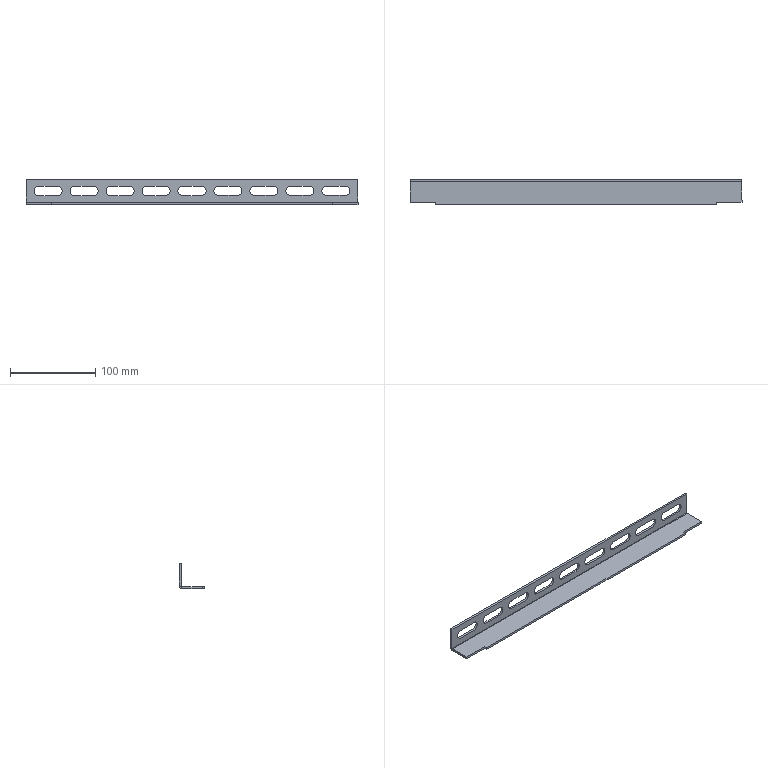Part | SolidWorks | features MirrorStock 1 | 1 solid | 63 faces | box 390 x 30 x 30 mm | volume 47297 mm3 | plane 34 | cylinder 29 | commonest cylinder face diameters 11 x27 1 x1 6 x1